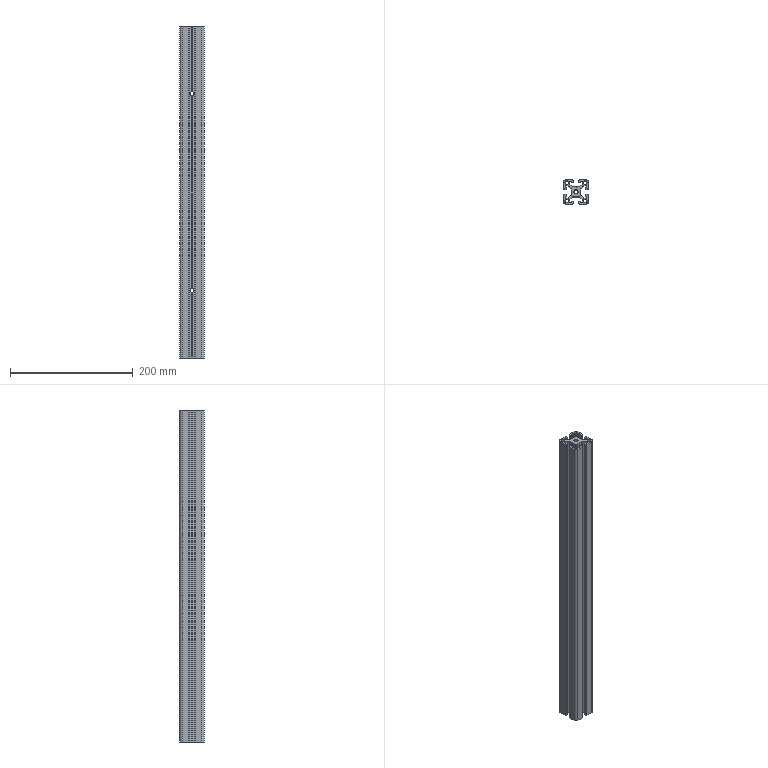Part | STEP file | HM-8-4040D-L540-machining required | 1 solid | 224 faces | box 40 x 40 x 540 mm | volume 368969 mm3 | cylinder 114 | plane 110 | commonest cylinder face diameters 1 x44 0.4 x36 4 x8 6 x8 6.6 x8 9 x4